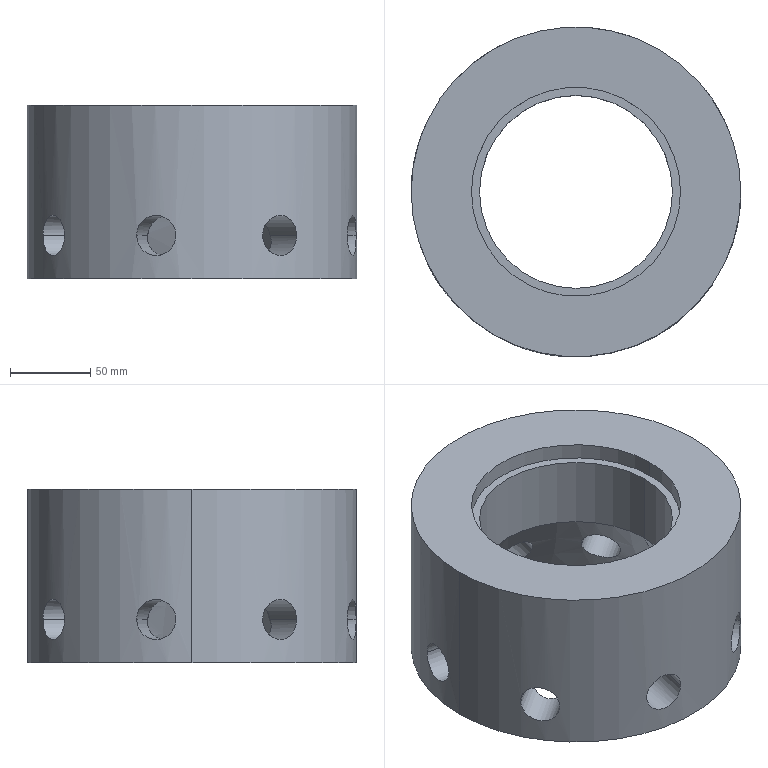Part | SolidWorks | features 3DProfileFeature 8, HoleWzd 8, RevCut 1, Revolution 1 | 1 solid | 27 faces | box 205 x 205 x 108 mm | volume 1920095 mm3 | cylinder 22 | plane 3 | cone 2 | commonest cylinder face diameters 25 x16 120 x2 130 x2 205 x2